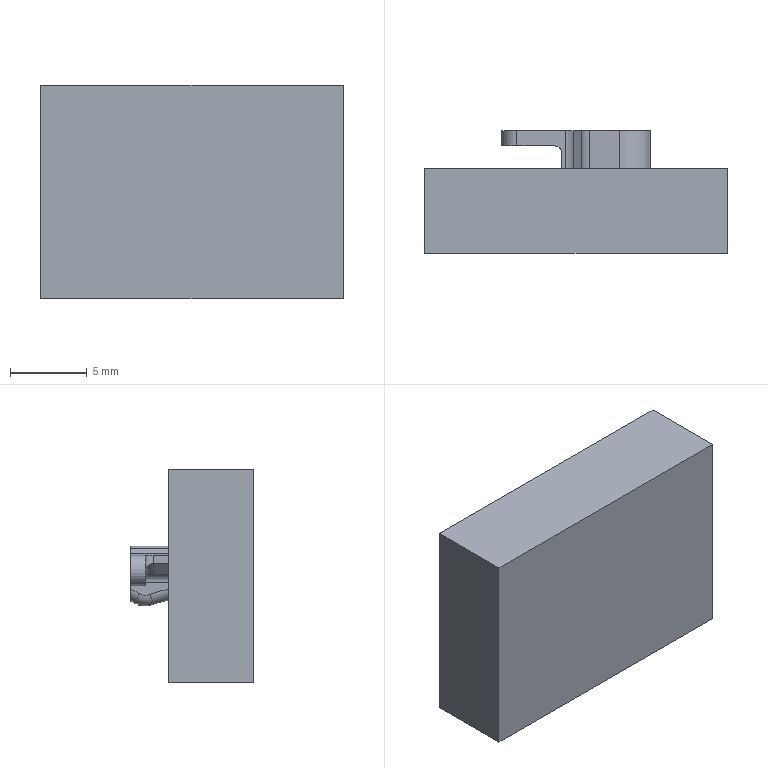NC program | NX | posted with a generic post | part box 19.7 x 8 x 13.91 mm
Lines 5587 to 6709 of 12456:
(CAVITY_MILL_COPY , TOOL : D1)
N11172 T05 M6
N11174 G54
N11176 G17 G0 G90 X5.779 Y0.829 B0. C0. S6000 M3
N11178 G43 Z30. H5
N11180 Z-1.065
N11182 G94 G1 Z-2.065 F1000.
N11184 G2 X5.966 Y1.183 R1.
N11186 G3 X6.079 Y1.5 R0.5 F850.
N11188 G1 X5.462
N11190 G3 X4.78 Y1.372 R1.743
N11192 G1 Y0.201
N11194 G3 X5.27 Y0.602 R0.5
N11196 G2 X5.678 Y1.01 R0.52
N11198 G3 X5.966 Y1.183 R0.5
N11200 G2 X6.434 Y1.36 R0.5
N11202 G1 X6.798 Y1.3
N11204 Z-1.065
N11206 G0 X5.812 Y0.829 Z-1.08
N11208 G1 Z-2.08 F1000.
N11210 G2 X5.998 Y1.183 R1.
N11212 G3 X6.111 Y1.5 R0.5 F850.
N11214 G1 X5.494
N11216 G3 X4.812 Y1.369 R1.793
N11218 G1 Y0.201
N11220 G3 X5.302 Y0.602 R0.5
N11222 G2 X5.71 Y1.01 R0.52
N11224 G3 X5.998 Y1.183 R0.5
N11226 G2 X6.466 Y1.36 R0.5
N11228 G1 X6.83 Y1.3
N11230 Z-1.08
N11232 G0 X5.844 Y0.829 Z-1.095
N11234 G1 Z-2.095 F1000.
N11236 G2 X6.03 Y1.183 R1.
N11238 G3 X6.143 Y1.5 R0.5 F850.
N11240 G1 X5.527
N11242 G3 X5.012 Y1.43 R2.66
N11244 G1 X4.922 Y1.415
N11246 X4.844 Y1.368
N11248 Y0.201
N11250 G3 X5.335 Y0.602 R0.5
N11252 G2 X5.742 Y1.01 R0.52
N11254 G3 X6.03 Y1.183 R0.5
N11256 G2 X6.498 Y1.36 R0.5
N11258 G1 X6.862 Y1.3
N11260 Z-1.095
N11262 G0 X5.876 Y0.829 Z-1.11
N11264 G1 Z-2.11 F1000.
N11266 G2 X6.062 Y1.183 R1.
N11268 G3 X6.175 Y1.5 R0.5 F850.
N11270 G1 X5.559
N11272 G3 X4.876 Y1.37 R1.927
N11274 G1 Y0.201
N11276 G3 X5.367 Y0.602 R0.5
N11278 G2 X5.774 Y1.01 R0.52
N11280 G3 X6.062 Y1.183 R0.5
N11282 G2 X6.53 Y1.36 R0.5
N11284 G1 X6.894 Y1.3
N11286 Z-1.11
N11288 G0 X5.908 Y0.829 Z-1.125
N11290 G1 Z-2.125 F1000.
N11292 G2 X6.094 Y1.183 R1.
N11294 G3 X6.208 Y1.5 R0.5 F850.
N11296 G1 X5.591
N11298 G3 X4.909 Y1.369 R1.869
N11300 G1 Y0.201
N11302 G3 X5.399 Y0.602 R0.5
N11304 G2 X5.806 Y1.01 R0.52
N11306 G3 X6.094 Y1.183 R0.5
N11308 G2 X6.562 Y1.36 R0.5
N11310 G1 X6.927 Y1.3
N11312 Z-1.125
N11314 G0 X5.94 Y0.829 Z-1.14
N11316 G1 Z-2.14 F1000.
N11318 G2 X6.127 Y1.183 R1.
N11320 G3 X6.24 Y1.5 R0.5 F850.
N11322 G1 X5.623
N11324 G3 X4.941 Y1.368 R1.908
N11326 G1 Y0.201
N11328 G3 X5.431 Y0.602 R0.5
N11330 G2 X5.838 Y1.01 R0.52
N11332 G3 X6.127 Y1.183 R0.5
N11334 G2 X6.594 Y1.36 R0.5
N11336 G1 X6.959 Y1.3
N11338 Z-1.14
N11340 G0 X5.972 Y0.829 Z-1.155
N11342 G1 Z-2.155 F1000.
N11344 G2 X6.159 Y1.183 R1.
N11346 G3 X6.272 Y1.5 R0.5 F850.
N11348 G1 X5.655
N11350 G3 X4.973 Y1.368 R1.841
N11352 G1 Y0.201
N11354 G3 X5.463 Y0.602 R0.5
N11356 G2 X5.87 Y1.01 R0.52
N11358 G3 X6.159 Y1.183 R0.5
N11360 G2 X6.626 Y1.36 R0.5
N11362 G1 X6.991 Y1.3
N11364 Z-1.155
N11366 G0 X5.921 Y0.809 Z-1.17
N11368 G1 Z-2.17 F1000.
N11370 G2 X6.15 Y1.139 R1.
N11372 G3 X6.289 Y1.38 R0.5 F850.
N11374 G1 Y1.48
N11376 X6.304
N11378 Y1.5
N11380 X5.687
N11382 G3 X5.107 Y1.408 R2.24
N11384 G1 X5.052 Y1.399
N11386 X5.005 Y1.367
N11388 Y0.201
N11390 G3 X5.495 Y0.602 R0.5
N11392 G2 X5.903 Y1.01 R0.52
N11394 G3 X6.15 Y1.139 R0.5
N11396 G2 X7.121 Y1.376 R1.
N11398 G1 X7.38 Y1.3
N11400 Z-1.17
N11402 G0 X5.872 Y0.774 Z-1.185
N11404 G1 Z-2.185 F1000.
N11406 G2 X6.145 Y1.107 R1.
N11408 G3 X6.289 Y1.289 R0.5 F850.
N11410 G1 Y1.48
N11412 X6.336 Y1.481
N11414 Y1.5
N11416 X5.719
N11418 G3 X5.037 Y1.366 R1.71
N11420 G1 Y0.201
N11422 G3 X5.527 Y0.602 R0.5
N11424 G2 X5.935 Y1.01 R0.52
N11426 G3 X6.145 Y1.107 R0.5
N11428 G2 X6.967 Y1.3 R1.
N11430 G1 Z-1.185
N11432 G0 X5.81 Y0.688 Z-1.2
N11434 G1 Z-2.2 F1000.
N11436 G2 X6.15 Y1.087 R1.
N11438 G3 X6.289 Y1.23 R0.5 F850.
N11440 G1 Y1.48
N11442 X6.368 Y1.481
N11444 Y1.5
N11446 X5.752
N11448 G3 X5.069 Y1.366 R1.615
N11450 G1 Y0.201
N11452 G3 X5.56 Y0.603 R0.5
N11454 G2 X5.967 Y1.01 R0.52
N11456 G3 X6.15 Y1.087 R0.5
N11458 G2 X6.815 Y1.257 R1.
N11460 G1 Z-1.2
N11462 G0 X5.682 Y0.31 Z-1.215
N11464 G1 Z-2.215 F1000.
N11466 G2 X6.16 Y1.072 R1.
N11468 G1 X6.236 Y1.116 F850.
N11470 X6.289 Y1.186
N11472 Y1.48
N11474 X6.4 Y1.482
N11476 Y1.5
N11478 X5.783
N11480 G3 X5.101 Y1.365 R1.617
N11482 G1 Y0.201
N11484 G3 X5.592 Y0.603 R0.5
N11486 G2 X5.999 Y1.01 R0.52
N11488 G1 X6.086 Y1.025
N11490 X6.16 Y1.072
N11492 G2 X6.818 Y1.207 R1.
N11494 G1 Z-1.215
N11496 G0 X5.648 Y0.226 Z-1.23
N11498 G1 Z-2.23 F1000.
N11500 G2 X6.171 Y1.06 R1.
N11502 G1 X6.239 Y1.093 F850.
N11504 X6.289 Y1.15
N11506 Y1.48
N11508 X6.432 Y1.482
N11510 X6.433 Y1.5
N11512 X5.783
N11514 G3 X5.134 Y1.364 R1.563
N11516 G1 Y0.201
N11518 G3 X5.624 Y0.602 R0.5
N11520 G2 X6.031 Y1.01 R0.52
N11522 G1 X6.106 Y1.02
N11524 X6.171 Y1.06
N11526 G2 X6.82 Y1.166 R1.
N11528 G1 Z-1.23
N11530 G0 X5.598 Y0.151 Z-1.245
N11532 G1 Z-2.245 F1000.
N11534 X5.605 Y0.227
N11536 G2 X6.177 Y1.047 R1.
N11538 G1 X6.241 Y1.071 F850.
N11540 X6.289 Y1.12
N11542 Y1.48
N11544 X6.415 Y1.482
N11546 X6.464
N11548 X6.465 Y1.5
N11550 X5.783
N11552 X5.766 Y1.493
N11554 X5.571 Y1.479
N11556 G3 X5.166 Y1.364 R1.04
N11558 G1 Y0.201
N11560 G3 X5.656 Y0.602 R0.5
N11562 G2 X6.063 Y1.01 R0.52
N11564 G1 X6.124 Y1.016
N11566 X6.177 Y1.047
N11568 G2 X6.809 Y1.12 R1.
N11570 G1 Z-1.245
N11572 G0 X5.538 Y0.089 Z-1.26
N11574 G1 Z-2.26 F1000.
N11576 X5.561 Y0.251
N11578 G2 X6.182 Y1.035 R1.
N11580 G1 X6.242 Y1.053 F850.
N11582 X6.289 Y1.094
N11584 Y1.48
N11586 X6.415 Y1.482
N11588 X6.497
N11590 Y1.5
N11592 X5.818
N11594 X5.801 Y1.496
N11596 X5.56 Y1.476
N11598 G3 X5.198 Y1.363 R0.959
N11600 G1 Y0.201
N11602 G3 X5.688 Y0.602 R0.5
N11604 G2 X6.095 Y1.01 R0.52
N11606 G1 X6.182 Y1.035
N11608 G2 X6.79 Y1.077 R1.
N11610 G1 Z-1.26
N11612 G0 X5.469 Y0.043 Z-1.275
N11614 G1 Z-2.275 F1000.
N11616 X5.518 Y0.28
N11618 G2 X6.185 Y1.025 R1.
N11620 G1 X6.243 Y1.037 F850.
N11622 X6.289 Y1.073
N11624 Y1.48
N11626 X6.415 Y1.482
N11628 X6.529
N11630 Y1.5
N11632 X5.853
N11634 X5.836 Y1.496
N11636 X5.624 Y1.478
N11638 X5.573 Y1.472
N11640 X5.292 Y1.398
N11642 X5.23 Y1.363
N11644 Y0.201
N11646 G3 X5.72 Y0.602 R0.5
N11648 G2 X6.128 Y1.01 R0.52
N11650 G1 X6.185 Y1.025
N11652 G2 X6.788 Y1.032 R1.
N11654 G1 Z-1.275
N11656 G0 X5.963 Y0.614 Z-1.29
N11658 G1 Z-2.29 F1000.
N11660 X5.831 Y0.665
N11662 G2 X6.187 Y1.016 R0.5
N11664 G1 X6.243 Y1.023 F850.
N11666 X6.289 Y1.055
N11668 Y1.48
N11670 X6.415 Y1.482
N11672 X6.561
N11674 Y1.5
N11676 X5.888
N11678 G3 X5.33 Y1.401 R2.258
N11680 G1 X5.262 Y1.362
N11682 Y0.201
N11684 G3 X5.752 Y0.602 R0.5
N11686 G2 X6.16 Y1.01 R0.52
N11688 G1 X6.187 Y1.016
N11690 G2 X6.785 Y0.987 R1.
N11692 G1 Z-1.29
N11694 G0 X5.994 Y0.611 Z-1.305
N11696 G1 Z-2.305 F1000.
N11698 X5.815 Y0.676
N11700 G2 X6.189 Y1.009 R0.5
N11702 G1 X6.192 Y1.01 F850.
N11704 X6.244 Y1.013
N11706 X6.289 Y1.04
N11708 Y1.48
N11710 X6.415 Y1.482
N11712 X6.593
N11714 Y1.5
N11716 X5.923
N11718 G3 X5.362 Y1.401 R2.232
N11720 G1 X5.294 Y1.361
N11722 Y0.201
N11724 G3 X5.785 Y0.602 R0.5
N11726 G2 X6.189 Y1.009 R0.52
N11728 X6.781 Y0.951 R1.
N11730 G1 Z-1.305
N11732 G0 X6.02 Y0.593 Z-1.32
N11734 G1 Z-2.32 F1000.
N11736 X5.838 Y0.648
N11738 G2 X6.191 Y1.002 R0.5
N11740 G1 X6.224 Y1.01 F850.
N11742 X6.289 Y1.028
N11744 Y1.48
N11746 X6.415 Y1.482
N11748 X6.625
N11750 Y1.5
N11752 X5.941
N11754 G3 X5.414 Y1.405 R2.132
N11756 G1 X5.364 Y1.396
N11758 X5.326 Y1.361
N11760 Y0.201
N11762 G3 X5.817 Y0.602 R0.5
N11764 G2 X6.191 Y1.002 R0.52
N11766 X6.787 Y0.979 R1.
N11768 G1 Z-1.32
N11770 G0 X5.606 Y0.046 Z-1.335
N11772 G1 Z-2.335 F1000.
N11774 X5.531 Y0.244
N11776 G2 X6.194 Y0.993 R1.
N11778 G1 X6.256 Y1.01 F850.
N11780 X6.289 Y1.018
N11782 Y1.48
N11784 X6.415 Y1.482
N11786 X6.657
N11788 X6.658 Y1.5
N11790 X5.976
N11792 G3 X5.456 Y1.407 R1.931
N11794 G1 X5.402 Y1.396
N11796 X5.359 Y1.361
N11798 Y0.201
N11800 G3 X5.849 Y0.602 R0.5
N11802 G2 X6.194 Y0.993 R0.52
N11804 X6.799 Y1.002 R1.
N11806 G1 Z-1.335
N11808 G0 X5.636 Y0.045 Z-1.35
N11810 G1 Z-2.35 F1000.
N11812 X5.579 Y0.197
N11814 G2 X6.198 Y0.983 R1.
N11816 G1 X6.289 Y1.01 F850.
N11818 Y1.48
N11820 X6.415 Y1.482
N11822 X6.689
N11824 X6.69 Y1.5
N11826 X6.007
N11828 G3 X5.458 Y1.401 R2.264
N11830 G1 X5.391 Y1.361
N11832 Y0.201
N11834 G3 X5.881 Y0.602 R0.5
N11836 G2 X6.198 Y0.983 R0.52
N11838 X6.859 Y1.011 R1.
N11840 G1 Z-1.35
N11842 G0 X5.67 Y0.046 Z-1.365
N11844 G1 Z-2.365 F1000.
N11846 X5.63 Y0.152
N11848 G2 X6.203 Y0.971 R1.
N11850 G1 X6.289 Y1.003 F850.
N11852 Y1.48
N11854 X6.415 Y1.482
N11856 X6.722
N11858 Y1.5
N11860 X6.105
N11862 G3 X5.49 Y1.401 R2.027
N11864 G1 X5.423 Y1.361
N11866 Y0.201
N11868 G3 X5.913 Y0.602 R0.5
N11870 G2 X6.203 Y0.971 R0.52
N11872 X6.917 Y1.022 R1.
N11874 G1 Z-1.365
N11876 G0 X5.679 Y0.038 Z-1.38
N11878 G1 Z-2.38 F1000.
N11880 X5.682 Y0.109
N11882 G2 X6.21 Y0.959 R1.
N11884 G1 X6.289 Y0.993 F850.
N11886 Y1.48
N11888 X6.415 Y1.482
N11890 X6.754
N11892 Y1.5
N11894 X6.137
N11896 G3 X5.522 Y1.401 R2.041
N11898 G1 X5.458 Y1.361
N11900 X5.455 Y1.351
N11902 Y0.201
N11904 G3 X5.945 Y0.602 R0.5
N11906 G2 X6.21 Y0.959 R0.52
N11908 X6.974 Y1.033 R1.
N11910 G1 Z-1.38
N11912 G0 X5.861 Y0.109 Z-1.395
N11914 G1 Z-2.395 F1000.
N11916 G2 X6.086 Y0.831 R1.
N11918 X6.289 Y0.981 R0.52 F850.
N11920 G1 Y1.48
N11922 X6.415 Y1.482
N11924 X6.786
N11926 Y1.5
N11928 X6.274
N11930 G3 X5.556 Y1.401 R2.201
N11932 G1 X5.49 Y1.361
N11934 X5.487 Y1.351
N11936 Y0.201
N11938 G3 X5.977 Y0.602 R0.5
N11940 G2 X6.086 Y0.831 R0.52
N11942 X7.023 Y1.181 R1.
N11944 G1 X7.166 Y1.157
N11946 Z-1.395
N11948 G0 X5.904 Y0.116 Z-1.41
N11950 G1 Z-2.41 F1000.
N11952 G2 X6.107 Y0.817 R1.
N11954 X6.289 Y0.966 R0.52 F850.
N11956 G1 Y1.48
N11958 X6.415 Y1.482
N11960 X6.818
N11962 Y1.5
N11964 X6.274
N11966 G3 X5.591 Y1.401 R2.169
N11968 G1 X5.522 Y1.362
N11970 X5.519 Y1.352
N11972 Y0.201
N11974 G3 X6.01 Y0.602 R0.5
N11976 G2 X6.107 Y0.817 R0.52
N11978 X7.031 Y1.199 R1.
N11980 G1 X7.213 Y1.175
N11982 Z-1.41
N11984 G0 X5.947 Y0.123 Z-1.425
N11986 G1 Z-2.425 F1000.
N11988 G2 X6.128 Y0.802 R1.
N11990 X6.289 Y0.949 R0.52 F850.
N11992 G1 Y1.48
N11994 X6.415 Y1.482
N11996 X6.85
N11998 Y1.5
N12000 X6.234
N12002 G3 X5.625 Y1.401 R2.166
N12004 G1 X5.554 Y1.362
N12006 X5.551 Y1.352
N12008 Y0.201
N12010 G3 X6.042 Y0.602 R0.5
N12012 G2 X6.128 Y0.802 R0.52
N12014 X7.039 Y1.216 R1.
N12016 G1 X7.26 Y1.195
N12018 Z-1.425
N12020 G0 X5.99 Y0.131 Z-1.44
N12022 G1 Z-2.44 F1000.
N12024 G2 X6.15 Y0.787 R1.
N12026 X6.289 Y0.929 R0.52 F850.
N12028 G1 Y1.48
N12030 X6.415 Y1.482
N12032 X6.882
N12034 X6.883 Y1.5
N12036 X6.266
N12038 X5.942 Y1.473
N12040 X5.836 Y1.454
N12042 G3 X5.584 Y1.352 R0.677
N12044 G1 Y0.201
N12046 G3 X6.074 Y0.602 R0.5
N12048 G2 X6.15 Y0.787 R0.52
N12050 X7.044 Y1.234 R1.
N12052 G1 X7.307 Y1.218
N12054 Z-1.44
N12056 G0 X6.032 Y0.139 Z-1.455
N12058 G1 Z-2.455 F1000.
N12060 G2 X6.171 Y0.77 R1.
N12062 G1 X6.217 Y0.849 F850.
N12064 X6.289 Y0.905
N12066 Y1.48
N12068 X6.415 Y1.482
N12070 X6.914
N12072 X6.915 Y1.5
N12074 X6.269
N12076 X5.977 Y1.474
N12078 G3 X5.616 Y1.353 R0.866
N12080 G1 Y0.201
N12082 G3 X6.106 Y0.602 R0.5
N12084 G1 X6.122 Y0.693
N12086 X6.171 Y0.77
N12088 G2 X7.048 Y1.251 R1.
N12090 G1 X7.354 Y1.244
N12092 Z-1.455
N12094 G0 X6.076 Y0.147 Z-1.47
N12096 G1 Z-2.47 F1000.
N12098 G2 X6.193 Y0.751 R1.
N12100 G1 X6.228 Y0.824 F850.
N12102 X6.289 Y0.877
N12104 Y1.48
N12106 X6.415 Y1.482
N12108 X6.947
N12110 Y1.5
N12112 X6.269
N12114 X6.021 Y1.474
N12116 G3 X5.648 Y1.354 R0.872
N12118 G1 Y0.201
N12120 G3 X6.138 Y0.602 R0.5
N12122 G1 X6.15 Y0.682
N12124 X6.193 Y0.751
N12126 G2 X7.049 Y1.268 R1.
N12128 G1 X7.402 Y1.275
N12130 Z-1.47
N12132 G0 X6.119 Y0.156 Z-1.485
N12134 G1 Z-2.485 F1000.
N12136 G2 X6.214 Y0.731 R1.
N12138 G1 X6.24 Y0.795 F850.
N12140 X6.289 Y0.843
N12142 Y1.48
N12144 X6.415 Y1.482
N12146 X6.979
N12148 Y1.5
N12150 X6.269
N12152 X6.017 Y1.471
N12154 G3 X5.68 Y1.355 R0.869
N12156 G1 Y0.201
N12158 G3 X6.17 Y0.602 R0.5
N12160 G1 X6.178 Y0.671
N12162 X6.214 Y0.731
N12164 G2 X7.046 Y1.285 R1.
N12166 G1 X7.141 Y1.009
N12168 Z-1.485
N12170 G0 X6.163 Y0.165 Z-1.5
N12172 G1 Z-2.5 F1000.
N12174 G2 X6.235 Y0.707 R1.
N12176 G1 X6.251 Y0.761 F850.
N12178 X6.289 Y0.803
N12180 Y1.48
N12182 X6.415 Y1.482
N12184 X7.011
N12186 Y1.5
N12188 X6.269
N12190 G3 X5.978 Y1.456 R36.635
N12192 G1 X5.926 Y1.444
N12194 X5.712 Y1.365
N12196 Y0.201
N12198 G3 X6.202 Y0.602 R0.5
N12200 G1 X6.206 Y0.659
N12202 X6.235 Y0.707
N12204 G2 X7.039 Y1.302 R1.
N12206 G1 X7.088 Y0.988
N12208 Z-1.5
N12210 G0 X6.208 Y0.176 Z-1.515
N12212 G1 Z-2.515 F1000.
N12214 G2 X6.256 Y0.679 R1.
N12216 G1 X6.289 Y0.752 F850.
N12218 Y1.48
N12220 X6.415 Y1.482
N12222 X7.043
N12224 Y1.5
N12226 X6.269
N12228 G3 X5.828 Y1.401 R2.197
N12230 G1 X5.746 Y1.367
N12232 X5.744 Y1.357
N12234 Y0.201
N12236 G3 X6.235 Y0.602 R0.5
N12238 G1 X6.256 Y0.679
N12240 G2 X7.024 Y1.32 R1.
N12242 G1 Y0.982
N12244 Z-1.515
N12246 G0 X6.614 Y0.302 Z-1.53
N12248 G1 Z-2.53 F1000.
N12250 G2 X6.289 Y1.04 R1.
N12252 G1 Y1.48 F850.
N12254 X6.415 Y1.482
N12256 X7.075
N12258 Y1.5
N12260 X6.269
N12262 G3 X5.779 Y1.368 R1.989
N12264 G1 X5.776 Y1.358
N12266 Y0.201
N12268 G3 X6.267 Y0.602 R0.5
N12270 G1 X6.289 Y0.682
N12272 Y1.04
N12274 G2 X6.539 Y1.473 R0.5
N12276 G1 X6.789 Y0.982
N12278 Z-1.53
N12280 G0 X6.678 Y0.248 Z-1.545
N12282 G1 Z-2.545 F1000.
N12284 G2 X6.289 Y1.04 R1.
N12286 G1 Y1.48 F850.
N12288 X6.415 Y1.482
N12290 X7.107
N12292 X7.108 Y1.5
N12294 X6.269
N12296 G3 X5.811 Y1.369 R2.122
N12298 G1 X5.809 Y1.359
N12300 Y0.201
N12302 G3 X6.289 Y0.563 R0.5
N12304 G1 Y1.04
N12306 G2 X6.539 Y1.473 R0.5
N12308 G1 X6.789 Y0.982
N12310 Z-1.545
N12312 G0 X6.716 Y0.22 Z-1.56
N12314 G1 Z-2.56 F1000.
N12316 G2 X6.289 Y1.04 R1.
N12318 G1 Y1.48 F850.
N12320 X6.415 Y1.482
N12322 X7.139
N12324 X7.14 Y1.5
N12326 X6.269
N12328 X5.921 Y1.401
N12330 X5.843 Y1.37
N12332 X5.841 Y1.36
N12334 Y0.201
N12336 G3 X6.289 Y0.48 R0.5
N12338 G1 Y1.04
N12340 G2 X6.539 Y1.473 R0.5
N12342 G1 X6.789 Y0.982
N12344 Z-1.56
N12346 G0 X6.739 Y0.205 Z-1.575
N12348 G1 Z-2.575 F1000.
N12350 G2 X6.289 Y1.04 R1.
N12352 G1 Y1.48 F850.
N12354 X6.415 Y1.482
N12356 X7.172
N12358 Y1.5
N12360 X6.269
N12362 G2 X5.951 Y1.401 R2.549
N12364 G1 X5.875 Y1.37
N12366 X5.873 Y1.36
N12368 Y0.201
N12370 G3 X6.289 Y0.424 R0.5
N12372 G1 Y1.04
N12374 G2 X6.539 Y1.473 R0.5
N12376 G1 X6.789 Y0.982
N12378 Z-1.575
N12380 G0 X6.753 Y0.195 Z-1.59
N12382 G1 Z-2.59 F1000.
N12384 G2 X6.289 Y1.04 R1.
N12386 G1 Y1.48 F850.
N12388 X6.415 Y1.482
N12390 X7.204
N12392 Y1.5
N12394 X6.269
N12396 G2 X5.981 Y1.401 R1.303
N12398 G1 X5.907 Y1.371
N12400 X5.905 Y1.361
N12402 Y0.201
N12404 G3 X6.289 Y0.381 R0.5
N12406 G1 Y1.04
N12408 G2 X6.539 Y1.473 R0.5
N12410 G1 X6.789 Y0.982
N12412 Z-1.59
N12414 G0 X6.764 Y0.189 Z-1.605
N12416 G1 Z-2.605 F1000.
N12418 G2 X6.289 Y1.04 R1.
N12420 G1 Y1.48 F850.
N12422 X6.415 Y1.482
N12424 X7.236
N12426 Y1.5
N12428 X6.269
N12430 G2 X5.994 Y1.394 R1.049
N12432 G1 X5.94 Y1.371
N12434 X5.937 Y1.361
N12436 Y0.201
N12438 G3 X6.289 Y0.346 R0.5
N12440 G1 Y1.04
N12442 G2 X6.539 Y1.473 R0.5
N12444 G1 X6.789 Y0.982
N12446 Z-1.605
N12448 G0 X6.771 Y0.184 Z-1.62
N12450 G1 Z-2.62 F1000.
N12452 G2 X6.289 Y1.04 R1.
N12454 G1 Y1.48 F850.
N12456 X6.415 Y1.482
N12458 X7.268
N12460 Y1.5
N12462 X6.269
N12464 G2 X6.039 Y1.401 R0.605
N12466 G1 X5.972 Y1.372
N12468 X5.969 Y1.362
N12470 Y0.201
N12472 G3 X6.289 Y0.317 R0.5
N12474 G1 Y1.04
N12476 G2 X6.539 Y1.473 R0.5
N12478 G1 X6.789 Y0.982
N12480 Z-1.62
N12482 G0 X6.777 Y0.181 Z-1.635
N12484 G1 Z-2.635 F1000.
N12486 G2 X6.289 Y1.04 R1.
N12488 G1 Y1.48 F850.
N12490 X6.415 Y1.482
N12492 X7.3
N12494 Y1.5
N12496 X6.269
N12498 X6.223 Y1.454
N12500 X6.165 Y1.423
N12502 X6.101 Y1.41
N12504 X6.068 Y1.401
N12506 X6.005 Y1.372
N12508 X6.001 Y1.362
N12510 Y0.201
N12512 G3 X6.289 Y0.292 R0.5
N12514 G1 Y1.04
N12516 G2 X6.539 Y1.473 R0.5
N12518 G1 X6.789 Y0.982
N12520 Z-1.635
N12522 G0 X6.781 Y0.179 Z-1.65
N12524 G1 Z-2.65 F1000.
N12526 G2 X6.289 Y1.04 R1.
N12528 G1 Y1.48 F850.
N12530 X6.415 Y1.482
N12532 X7.332
N12534 X7.333 Y1.5
N12536 X6.269
N12538 G2 X6.034 Y1.362 R1.469
N12540 G1 Y0.201
N12542 G3 X6.289 Y0.271 R0.5
N12544 G1 Y1.04
N12546 G2 X6.539 Y1.473 R0.5
N12548 G1 X6.789 Y0.982
N12550 Z-1.65
N12552 G0 X6.783 Y0.177 Z-1.665
N12554 G1 Z-2.665 F1000.
N12556 G2 X6.289 Y1.04 R1.
N12558 G1 Y1.48 F850.
N12560 X6.415 Y1.482
N12562 X7.364
N12564 X7.365 Y1.5
N12566 X6.269
N12568 G2 X6.066 Y1.363 R1.216
N12570 G1 Y0.201
N12572 G3 X6.289 Y0.254 R0.5
N12574 G1 Y1.04
N12576 G2 X6.539 Y1.473 R0.5
N12578 G1 X6.789 Y0.982
N12580 Z-1.665
N12582 G0 X6.785 Y0.176 Z-1.68
N12584 G1 Z-2.68 F1000.
N12586 G2 X6.289 Y1.04 R1.
N12588 G1 Y1.48 F850.
N12590 X6.415 Y1.482
N12592 X7.397
N12594 Y1.5
N12596 X6.269
N12598 X6.243 Y1.471
N12600 X6.098 Y1.363
N12602 Y0.201
N12604 X6.197
N12606 X6.289 Y0.239
N12608 Y1.04
N12610 G2 X6.539 Y1.473 R0.5
N12612 G1 X6.789 Y0.982
N12614 Z-1.68
N12616 G0 X6.787 Y0.175 Z-1.695
N12618 G1 Z-2.695 F1000.
N12620 G2 X6.289 Y1.04 R1.
N12622 G1 Y1.48 F850.
N12624 X6.415 Y1.482
N12626 X7.429
N12628 Y1.5
N12630 X6.269
N12632 X6.237 Y1.444
N12634 X6.189 Y1.4
N12636 X6.13 Y1.374
N12638 Y0.201
N12640 X6.212 Y0.198
N12642 X6.289 Y0.227
N12644 Y1.04
N12646 G2 X6.539 Y1.473 R0.5
N12648 G1 X6.789 Y0.982
N12650 Z-1.695
N12652 G0 X6.787 Y0.175 Z-1.71
N12654 G1 Z-2.71 F1000.
N12656 G2 X6.289 Y1.04 R1.
N12658 G1 Y1.48 F850.
N12660 X6.415 Y1.482
N12662 X7.461
N12664 Y1.5
N12666 X6.269
N12668 X6.187 Y1.399
N12670 X6.162 Y1.378
N12672 Y0.201
N12674 X6.228 Y0.195
N12676 X6.289 Y0.217
N12678 Y1.04
N12680 G2 X6.539 Y1.473 R0.5
N12682 G1 X6.789 Y0.982
N12684 Z-1.71
N12686 G0 X6.788 Y0.174 Z-1.725
N12688 G1 Z-2.725 F1000.
N12690 G2 X6.289 Y1.04 R1.
N12692 G1 Y1.48 F850.
N12694 X6.415 Y1.482
N12696 X7.493
N12698 Y1.5
N12700 X6.269
N12702 X6.194 Y1.384
N12704 Y0.201
N12706 X6.289 Y0.21
N12708 Y1.04
N12710 G2 X6.539 Y1.473 R0.5
N12712 G1 X6.789 Y0.982
N12714 Z-1.725
N12716 G0 X6.788 Y0.174 Z-1.74
N12718 G1 Z-2.74 F1000.
N12720 G2 X6.289 Y1.04 R1.
N12722 G1 Y1.48 F850.
N12724 X6.415 Y1.482
N12726 X7.525
N12728 Y1.5
N12730 X6.269
N12732 X6.259 Y1.471
N12734 X6.226 Y1.405
N12736 Y0.201
N12738 X6.289 Y0.205
N12740 Y1.04
N12742 G2 X6.539 Y1.473 R0.5
N12744 G1 X6.789 Y0.982
N12746 Z-1.74
N12748 G0 Y0.174 Z-1.755
N12750 G1 Z-2.755 F1000.
N12752 G2 X6.289 Y1.04 R1.
N12754 G1 Y1.48 F850.
N12756 X6.415 Y1.482
N12758 X7.557
N12760 X7.558 Y1.5
N12762 X6.269
N12764 X6.259 Y1.471
N12766 Y0.201
N12768 X6.289 Y0.202
N12770 Y1.04
N12772 G2 X6.539 Y1.473 R0.5
N12774 G1 X6.789 Y0.982
N12776 Z-1.755
N12778 G0 Y0.174 Z-1.77
N12780 G1 Z-2.77 F1000.
N12782 G2 X6.289 Y1.04 R1.
N12784 G1 Y1.48 F850.
N12786 X6.415 Y1.482
N12788 X7.568
N12790 Y1.5
N12792 X6.269
N12794 Y0.201
N12796 X6.289
N12798 Y1.04
N12800 G2 X6.539 Y1.473 R0.5
N12802 G1 X6.789 Y0.982
N12804 Z-1.77
N12806 G0 Y0.174 Z-1.785
N12808 G1 Z-2.785 F1000.
N12810 G2 X6.289 Y1.04 R1.
N12812 G1 Y1.48 F850.
N12814 X6.415 Y1.482
N12816 X7.568
N12818 Y1.5
N12820 X6.269
N12822 Y0.201
N12824 X6.289
N12826 Y1.04
N12828 G2 X6.539 Y1.473 R0.5
N12830 G1 X6.789 Y0.982
N12832 Z-1.785
N12834 G0 Y0.174 Z-1.8
N12836 G1 Z-2.8 F1000.
N12838 G2 X6.289 Y1.04 R1.
N12840 G1 Y1.48 F850.
N12842 X6.415 Y1.482
N12844 X7.568
N12846 Y1.5
N12848 X6.269
N12850 Y0.201
N12852 X6.289
N12854 Y1.04
N12856 G2 X6.539 Y1.473 R0.5
N12858 G1 X6.789 Y0.982
N12860 Z-1.8
N12862 G0 Y0.174 Z-1.815
N12864 G1 Z-2.815 F1000.
N12866 G2 X6.289 Y1.04 R1.
N12868 G1 Y1.48 F850.
N12870 X6.415 Y1.482
N12872 X7.568
N12874 Y1.5
N12876 X6.269
N12878 Y0.201
N12880 X6.289
N12882 Y1.04
N12884 G2 X6.539 Y1.473 R0.5
N12886 G1 X6.789 Y0.982
N12888 Z-1.815
N12890 G0 Y0.174 Z-1.83
N12892 G1 Z-2.83 F1000.
N12894 G2 X6.289 Y1.04 R1.
N12896 G1 Y1.48 F850.
N12898 X6.415 Y1.482
N12900 X7.568
N12902 Y1.5
N12904 X6.269
N12906 Y0.201
N12908 X6.289
N12910 Y1.04
N12912 G2 X6.539 Y1.473 R0.5
N12914 G1 X6.789 Y0.982
N12916 Z-1.83
N12918 G0 Y0.174 Z-1.845
N12920 G1 Z-2.845 F1000.
N12922 G2 X6.289 Y1.04 R1.
N12924 G1 Y1.48 F850.
N12926 X6.415 Y1.482
N12928 X7.568
N12930 Y1.5
N12932 X6.269
N12934 Y0.201
N12936 X6.289
N12938 Y1.04
N12940 G2 X6.539 Y1.473 R0.5
N12942 G1 X6.789 Y0.982
N12944 Z-1.845
N12946 G0 Y0.174 Z-1.86
N12948 G1 Z-2.86 F1000.
N12950 G2 X6.289 Y1.04 R1.
N12952 G1 Y1.48 F850.
N12954 X6.415 Y1.482
N12956 X7.568
N12958 Y1.5
N12960 X6.269
N12962 Y0.201
N12964 X6.289
N12966 Y1.04
N12968 G2 X6.539 Y1.473 R0.5
N12970 G1 X6.789 Y0.982
N12972 Z-1.86
N12974 G0 Y0.174 Z-1.875
N12976 G1 Z-2.875 F1000.
N12978 G2 X6.289 Y1.04 R1.
N12980 G1 Y1.48 F850.
N12982 X6.415 Y1.482
N12984 X7.568
N12986 Y1.5
N12988 X6.269
N12990 Y0.201
N12992 X6.289
N12994 Y1.04
N12996 G2 X6.539 Y1.473 R0.5
N12998 G1 X6.789 Y0.982
N13000 Z-1.875
N13002 G0 Y0.174 Z-1.89
N13004 G1 Z-2.89 F1000.
N13006 G2 X6.289 Y1.04 R1.
N13008 G1 Y1.48 F850.
N13010 X6.415 Y1.482
N13012 X7.568
N13014 Y1.5
N13016 X6.269
N13018 Y0.201
N13020 X6.289
N13022 Y1.04
N13024 G2 X6.539 Y1.473 R0.5
N13026 G1 X6.789 Y0.982
N13028 Z-1.89
N13030 G0 Y0.174 Z-1.905
N13032 G1 Z-2.905 F1000.
N13034 G2 X6.289 Y1.04 R1.
N13036 G1 Y1.48 F850.
N13038 X6.415 Y1.482
N13040 X7.568
N13042 Y1.5
N13044 X6.269
N13046 Y0.201
N13048 X6.289
N13050 Y1.04
N13052 G2 X6.539 Y1.473 R0.5
N13054 G1 X6.789 Y0.982
N13056 Z-1.905
N13058 G0 Y0.174 Z-1.92
N13060 G1 Z-2.92 F1000.
N13062 G2 X6.289 Y1.04 R1.
N13064 G1 Y1.48 F850.
N13066 X6.415 Y1.482
N13068 X7.568
N13070 Y1.5
N13072 X6.269
N13074 Y0.201
N13076 X6.289
N13078 Y1.04
N13080 G2 X6.539 Y1.473 R0.5
N13082 G1 X6.789 Y0.982
N13084 Z-1.92
N13086 G0 Y0.174 Z-1.935
N13088 G1 Z-2.935 F1000.
N13090 G2 X6.289 Y1.04 R1.
N13092 G1 Y1.48 F850.
N13094 X6.415 Y1.482
N13096 X7.568
N13098 Y1.5
N13100 X6.269
N13102 Y0.201
N13104 X6.289
N13106 Y1.04
N13108 G2 X6.539 Y1.473 R0.5
N13110 G1 X6.789 Y0.982
N13112 Z-1.935
N13114 G0 Y0.174 Z-1.95
N13116 G1 Z-2.95 F1000.
N13118 G2 X6.289 Y1.04 R1.
N13120 G1 Y1.48 F850.
N13122 X6.415 Y1.482
N13124 X7.568
N13126 Y1.5
N13128 X6.269
N13130 Y0.201
N13132 X6.289
N13134 Y1.04
N13136 G2 X6.539 Y1.473 R0.5
N13138 G1 X6.789 Y0.982
N13140 Z-1.95
N13142 G0 Y0.174 Z-1.965
N13144 G1 Z-2.965 F1000.
N13146 G2 X6.289 Y1.04 R1.
N13148 G1 Y1.48 F850.
N13150 X6.415 Y1.482
N13152 X7.568
N13154 Y1.5
N13156 X6.269
N13158 Y0.201
N13160 X6.289
N13162 Y1.04
N13164 G2 X6.539 Y1.473 R0.5
N13166 G1 X6.789 Y0.982
N13168 Z-1.965
N13170 G0 Y0.174 Z-1.98
N13172 G1 Z-2.98 F1000.
N13174 G2 X6.289 Y1.04 R1.
N13176 G1 Y1.48 F850.
N13178 X6.415 Y1.482
N13180 X7.568
N13182 Y1.5
N13184 X6.269
N13186 Y0.201
N13188 X6.289
N13190 Y1.04
N13192 G2 X6.539 Y1.473 R0.5
N13194 G1 X6.789 Y0.982
N13196 Z-1.98
N13198 G0 Y0.174 Z-1.995
N13200 G1 Z-2.995 F1000.
N13202 G2 X6.289 Y1.04 R1.
N13204 G1 Y1.48 F850.
N13206 X6.415 Y1.482
N13208 X7.568
N13210 Y1.5
N13212 X6.269
N13214 Y0.201
N13216 X6.289
N13218 Y1.04
N13220 G2 X6.539 Y1.473 R0.5
N13222 G1 X6.789 Y0.982
N13224 Z-1.995
N13226 G0 Y0.174 Z-2.01
N13228 G1 Z-3.01 F1000.
N13230 G2 X6.289 Y1.04 R1.
N13232 G1 Y1.48 F850.
N13234 X6.415 Y1.482
N13236 X7.568
N13238 Y1.5
N13240 X6.269
N13242 Y0.201
N13244 X6.289
N13246 Y1.04
N13248 G2 X6.539 Y1.473 R0.5
N13250 G1 X6.789 Y0.982
N13252 Z-2.01
N13254 G0 Y0.174 Z-2.025
N13256 G1 Z-3.025 F1000.
N13258 G2 X6.289 Y1.04 R1.
N13260 G1 Y1.48 F850.
N13262 X6.415 Y1.482
N13264 X7.568
N13266 Y1.5
N13268 X6.269
N13270 Y0.201
N13272 X6.289
N13274 Y1.04
N13276 G2 X6.539 Y1.473 R0.5
N13278 G1 X6.789 Y0.982
N13280 Z-2.025
N13282 G0 Y0.174 Z-2.04
N13284 G1 Z-3.04 F1000.
N13286 G2 X6.289 Y1.04 R1.
N13288 G1 Y1.48 F850.
N13290 X6.415 Y1.482
N13292 X7.568
N13294 Y1.5
N13296 X6.269
N13298 Y0.201
N13300 X6.289
N13302 Y1.04
N13304 G2 X6.539 Y1.473 R0.5
N13306 G1 X6.789 Y0.982
N13308 Z-2.04
N13310 G0 Y0.174 Z-2.055
N13312 G1 Z-3.055 F1000.
N13314 G2 X6.289 Y1.04 R1.
N13316 G1 Y1.48 F850.
N13318 X6.415 Y1.482
N13320 X7.568
N13322 Y1.5
N13324 X6.269
N13326 Y0.201
N13328 X6.289
N13330 Y1.04
N13332 G2 X6.539 Y1.473 R0.5
N13334 G1 X6.789 Y0.982
N13336 Z-2.055
N13338 G0 Y0.174 Z-2.07
N13340 G1 Z-3.07 F1000.
N13342 G2 X6.289 Y1.04 R1.
N13344 G1 Y1.48 F850.
N13346 X6.415 Y1.482
N13348 X7.568
N13350 Y1.5
N13352 X6.269
N13354 Y0.201
N13356 X6.289
N13358 Y1.04
N13360 G2 X6.539 Y1.473 R0.5
N13362 G1 X6.789 Y0.982
N13364 Z-2.07
N13366 G0 Y0.174 Z-2.085
N13368 G1 Z-3.085 F1000.
N13370 G2 X6.289 Y1.04 R1.
N13372 G1 Y1.48 F850.
N13374 X6.415 Y1.482
N13376 X7.568
N13378 Y1.5
N13380 X6.269
N13382 Y0.201
N13384 X6.289
N13386 Y1.04
N13388 G2 X6.539 Y1.473 R0.5
N13390 G1 X6.789 Y0.982
N13392 Z-2.085
N13394 G0 Y0.174 Z-2.1
N13396 G1 Z-3.1 F1000.
N13398 G2 X6.289 Y1.04 R1.
N13400 G1 Y1.48 F850.
N13402 X6.415 Y1.482
N13404 X7.568
N13406 Y1.5
N13408 X6.269
N13410 Y0.201